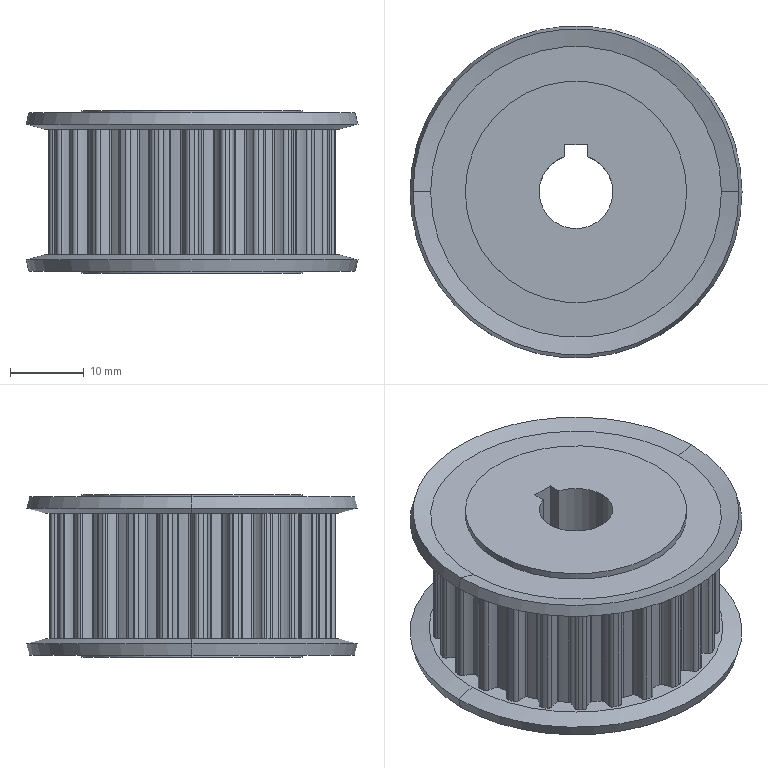Part | SolidWorks | features ICE 4, BaseBody 1 | 1 solid | 249 faces | box 45 x 45 x 22 mm | volume 22602 mm3 | cylinder 228 | cone 12 | plane 9 | commonest cylinder face diameters 1.1 x61 0.5 x57 6.55 x53 35.29 x25 38.83 x25 30 x4